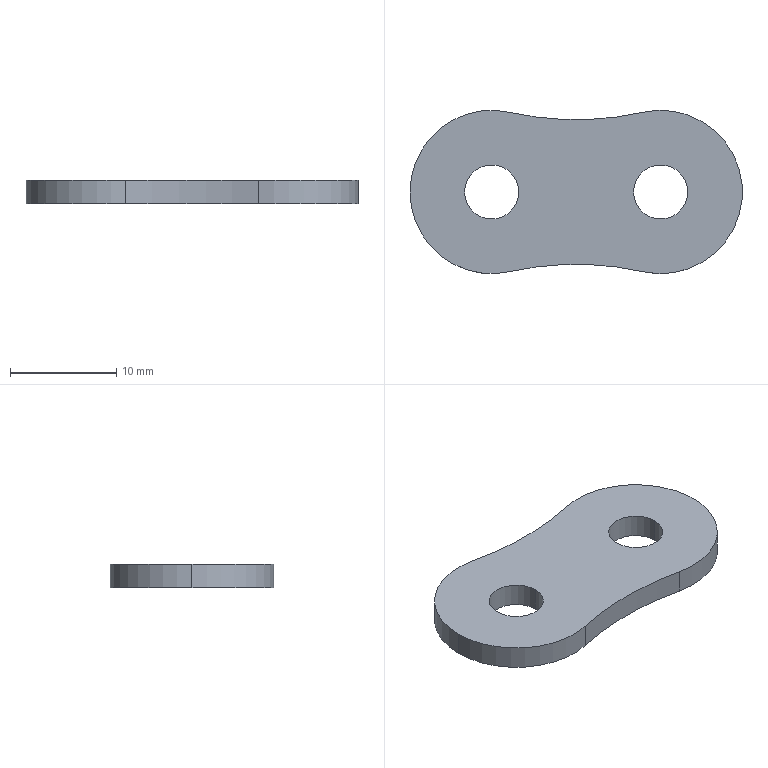Part | NX | features BREP 1 | 1 solid | 11 faces | box 31.225 x 15.35 x 2.22 mm | volume 824.256 mm3 | cylinder 9 | plane 2 | commonest cylinder face diameters 5.09 x4 15.35 x3 56.766 x2
STEP:
#1=CARTESIAN_POINT('',(5.393,0.,0.));
#2=VERTEX_POINT('',#1);
#3=CARTESIAN_POINT('',(10.482,0.,0.));
#4=VERTEX_POINT('',#3);
#5=CARTESIAN_POINT('',(7.938,0.,0.));
#6=DIRECTION('',(0.,0.,1.));
#7=DIRECTION('',(1.,0.,0.));
#8=AXIS2_PLACEMENT_3D('',#5,#6,#7);
#9=CIRCLE('',#8,2.545);
#10=EDGE_CURVE('',#2,#4,#9,.T.);
#11=ORIENTED_EDGE('',*,*,#10,.F.);
#12=CARTESIAN_POINT('',(5.393,0.,2.22));
#13=VERTEX_POINT('',#12);
#14=CARTESIAN_POINT('',(5.393,0.,0.));
#15=DIRECTION('',(0.,0.,1.));
#16=VECTOR('',#15,1000.);
#17=LINE('',#14,#16);
#18=EDGE_CURVE('',#13,#2,#17,.F.);
#19=ORIENTED_EDGE('',*,*,#18,.F.);
#20=CARTESIAN_POINT('',(10.482,0.,2.22));
#21=VERTEX_POINT('',#20);
#22=CARTESIAN_POINT('',(7.938,0.,2.22));
#23=DIRECTION('',(0.,0.,1.));
#24=DIRECTION('',(1.,0.,0.));
#25=AXIS2_PLACEMENT_3D('',#22,#23,#24);
#26=CIRCLE('',#25,2.545);
#27=EDGE_CURVE('',#13,#21,#26,.T.);
#28=ORIENTED_EDGE('',*,*,#27,.T.);
#29=CARTESIAN_POINT('',(10.482,0.,0.));
#30=DIRECTION('',(0.,0.,1.));
#31=VECTOR('',#30,1000.);
#32=LINE('',#29,#31);
#33=EDGE_CURVE('',#21,#4,#32,.F.);
#34=ORIENTED_EDGE('',*,*,#33,.T.);
#35=EDGE_LOOP('',(#11,#19,#28,#34));
#36=FACE_BOUND('',#35,.T.);
#37=CARTESIAN_POINT('',(7.938,0.,0.));
#38=DIRECTION('',(0.,0.,1.));
#39=DIRECTION('',(1.,0.,0.));
#40=AXIS2_PLACEMENT_3D('',#37,#38,#39);
#41=CYLINDRICAL_SURFACE('',#40,2.545);
#42=ADVANCED_FACE('',(#36),#41,.F.);
#43=CARTESIAN_POINT('',(-10.482,0.,0.));
#44=VERTEX_POINT('',#43);
#45=CARTESIAN_POINT('',(-5.393,0.,0.));
#46=VERTEX_POINT('',#45);
#47=CARTESIAN_POINT('',(-7.938,0.,0.));
#48=DIRECTION('',(0.,0.,1.));
#49=DIRECTION('',(1.,0.,0.));
#50=AXIS2_PLACEMENT_3D('',#47,#48,#49);
#51=CIRCLE('',#50,2.545);
#52=EDGE_CURVE('',#44,#46,#51,.T.);
#53=ORIENTED_EDGE('',*,*,#52,.F.);
#54=CARTESIAN_POINT('',(-10.482,0.,2.22));
#55=VERTEX_POINT('',#54);
#56=CARTESIAN_POINT('',(-10.482,0.,0.));
#57=DIRECTION('',(0.,0.,1.));
#58=VECTOR('',#57,1000.);
#59=LINE('',#56,#58);
#60=EDGE_CURVE('',#55,#44,#59,.F.);
#61=ORIENTED_EDGE('',*,*,#60,.F.);
#62=CARTESIAN_POINT('',(-5.393,0.,2.22));
#63=VERTEX_POINT('',#62);
#64=CARTESIAN_POINT('',(-7.938,0.,2.22));
#65=DIRECTION('',(0.,0.,1.));
#66=DIRECTION('',(1.,0.,0.));
#67=AXIS2_PLACEMENT_3D('',#64,#65,#66);
#68=CIRCLE('',#67,2.545);
#69=EDGE_CURVE('',#55,#63,#68,.T.);
#70=ORIENTED_EDGE('',*,*,#69,.T.);
#71=CARTESIAN_POINT('',(-5.393,0.,0.));
#72=DIRECTION('',(0.,0.,1.));
#73=VECTOR('',#72,1000.);
#74=LINE('',#71,#73);
#75=EDGE_CURVE('',#63,#46,#74,.F.);
#76=ORIENTED_EDGE('',*,*,#75,.T.);
#77=EDGE_LOOP('',(#53,#61,#70,#76));
#78=FACE_BOUND('',#77,.T.);
#79=CARTESIAN_POINT('',(-7.938,0.,0.));
#80=DIRECTION('',(0.,0.,1.));
#81=DIRECTION('',(1.,0.,0.));
#82=AXIS2_PLACEMENT_3D('',#79,#80,#81);
#83=CYLINDRICAL_SURFACE('',#82,2.545);
#84=ADVANCED_FACE('',(#78),#83,.F.);
#85=CARTESIAN_POINT('',(-15.613,0.,2.22));
#86=VERTEX_POINT('',#85);
#87=CARTESIAN_POINT('',(-6.248,-7.487,2.22));
#88=VERTEX_POINT('',#87);
#89=CARTESIAN_POINT('',(-7.938,0.,2.22));
#90=DIRECTION('',(0.,0.,1.));
#91=DIRECTION('',(1.,0.,0.));
#92=AXIS2_PLACEMENT_3D('',#89,#90,#91);
#93=CIRCLE('',#92,7.675);
#94=EDGE_CURVE('',#86,#88,#93,.T.);
#95=ORIENTED_EDGE('',*,*,#94,.F.);
#96=CARTESIAN_POINT('',(-15.613,0.,0.));
#97=VERTEX_POINT('',#96);
#98=CARTESIAN_POINT('',(-15.613,0.,2.22));
#99=DIRECTION('',(0.,0.,-1.));
#100=VECTOR('',#99,1000.);
#101=LINE('',#98,#100);
#102=EDGE_CURVE('',#86,#97,#101,.T.);
#103=ORIENTED_EDGE('',*,*,#102,.T.);
#104=CARTESIAN_POINT('',(-6.248,-7.487,0.));
#105=VERTEX_POINT('',#104);
#106=CARTESIAN_POINT('',(-7.938,0.,0.));
#107=DIRECTION('',(0.,0.,1.));
#108=DIRECTION('',(1.,0.,0.));
#109=AXIS2_PLACEMENT_3D('',#106,#107,#108);
#110=CIRCLE('',#109,7.675);
#111=EDGE_CURVE('',#97,#105,#110,.T.);
#112=ORIENTED_EDGE('',*,*,#111,.T.);
#113=CARTESIAN_POINT('',(-6.248,-7.487,2.22));
#114=DIRECTION('',(0.,0.,-1.));
#115=VECTOR('',#114,1000.);
#116=LINE('',#113,#115);
#117=EDGE_CURVE('',#88,#105,#116,.T.);
#118=ORIENTED_EDGE('',*,*,#117,.F.);
#119=EDGE_LOOP('',(#95,#103,#112,#118));
#120=FACE_BOUND('',#119,.T.);
#121=CARTESIAN_POINT('',(-7.938,0.,2.22));
#122=DIRECTION('',(0.,0.,-1.));
#123=DIRECTION('',(-1.,0.,0.));
#124=AXIS2_PLACEMENT_3D('',#121,#122,#123);
#125=CYLINDRICAL_SURFACE('',#124,7.675);
#126=ADVANCED_FACE('',(#120),#125,.T.);
#127=CARTESIAN_POINT('',(6.248,-7.487,0.));
#128=VERTEX_POINT('',#127);
#129=CARTESIAN_POINT('',(0.,-35.173,0.));
#130=DIRECTION('',(0.,0.,-1.));
#131=DIRECTION('',(1.,0.,0.));
#132=AXIS2_PLACEMENT_3D('',#129,#130,#131);
#133=CIRCLE('',#132,28.383);
#134=EDGE_CURVE('',#105,#128,#133,.T.);
#135=ORIENTED_EDGE('',*,*,#134,.T.);
#136=CARTESIAN_POINT('',(6.248,-7.487,2.22));
#137=VERTEX_POINT('',#136);
#138=CARTESIAN_POINT('',(6.248,-7.487,2.22));
#139=DIRECTION('',(0.,0.,-1.));
#140=VECTOR('',#139,1000.);
#141=LINE('',#138,#140);
#142=EDGE_CURVE('',#137,#128,#141,.T.);
#143=ORIENTED_EDGE('',*,*,#142,.F.);
#144=CARTESIAN_POINT('',(0.,-35.173,2.22));
#145=DIRECTION('',(0.,0.,-1.));
#146=DIRECTION('',(1.,0.,0.));
#147=AXIS2_PLACEMENT_3D('',#144,#145,#146);
#148=CIRCLE('',#147,28.383);
#149=EDGE_CURVE('',#88,#137,#148,.T.);
#150=ORIENTED_EDGE('',*,*,#149,.F.);
#151=ORIENTED_EDGE('',*,*,#117,.T.);
#152=EDGE_LOOP('',(#135,#143,#150,#151));
#153=FACE_BOUND('',#152,.T.);
#154=CARTESIAN_POINT('',(0.,-35.173,2.22));
#155=DIRECTION('',(0.,0.,-1.));
#156=DIRECTION('',(-1.,0.,0.));
#157=AXIS2_PLACEMENT_3D('',#154,#155,#156);
#158=CYLINDRICAL_SURFACE('',#157,28.383);
#159=ADVANCED_FACE('',(#153),#158,.F.);
#160=CARTESIAN_POINT('',(6.248,7.487,0.));
#161=VERTEX_POINT('',#160);
#162=CARTESIAN_POINT('',(7.938,0.,0.));
#163=DIRECTION('',(0.,0.,1.));
#164=DIRECTION('',(1.,0.,0.));
#165=AXIS2_PLACEMENT_3D('',#162,#163,#164);
#166=CIRCLE('',#165,7.675);
#167=EDGE_CURVE('',#128,#161,#166,.T.);
#168=ORIENTED_EDGE('',*,*,#167,.T.);
#169=CARTESIAN_POINT('',(6.248,7.487,2.22));
#170=VERTEX_POINT('',#169);
#171=CARTESIAN_POINT('',(6.248,7.487,2.22));
#172=DIRECTION('',(0.,0.,-1.));
#173=VECTOR('',#172,1000.);
#174=LINE('',#171,#173);
#175=EDGE_CURVE('',#170,#161,#174,.T.);
#176=ORIENTED_EDGE('',*,*,#175,.F.);
#177=CARTESIAN_POINT('',(7.938,0.,2.22));
#178=DIRECTION('',(0.,0.,1.));
#179=DIRECTION('',(1.,0.,0.));
#180=AXIS2_PLACEMENT_3D('',#177,#178,#179);
#181=CIRCLE('',#180,7.675);
#182=EDGE_CURVE('',#137,#170,#181,.T.);
#183=ORIENTED_EDGE('',*,*,#182,.F.);
#184=ORIENTED_EDGE('',*,*,#142,.T.);
#185=EDGE_LOOP('',(#168,#176,#183,#184));
#186=FACE_BOUND('',#185,.T.);
#187=CARTESIAN_POINT('',(7.938,0.,2.22));
#188=DIRECTION('',(0.,0.,-1.));
#189=DIRECTION('',(-1.,0.,0.));
#190=AXIS2_PLACEMENT_3D('',#187,#188,#189);
#191=CYLINDRICAL_SURFACE('',#190,7.675);
#192=ADVANCED_FACE('',(#186),#191,.T.);
#193=CARTESIAN_POINT('',(-6.248,7.487,0.));
#194=VERTEX_POINT('',#193);
#195=CARTESIAN_POINT('',(0.,35.173,0.));
#196=DIRECTION('',(0.,0.,-1.));
#197=DIRECTION('',(1.,0.,0.));
#198=AXIS2_PLACEMENT_3D('',#195,#196,#197);
#199=CIRCLE('',#198,28.383);
#200=EDGE_CURVE('',#161,#194,#199,.T.);
#201=ORIENTED_EDGE('',*,*,#200,.T.);
#202=CARTESIAN_POINT('',(-6.248,7.487,2.22));
#203=VERTEX_POINT('',#202);
#204=CARTESIAN_POINT('',(-6.248,7.487,2.22));
#205=DIRECTION('',(0.,0.,-1.));
#206=VECTOR('',#205,1000.);
#207=LINE('',#204,#206);
#208=EDGE_CURVE('',#203,#194,#207,.T.);
#209=ORIENTED_EDGE('',*,*,#208,.F.);
#210=CARTESIAN_POINT('',(0.,35.173,2.22));
#211=DIRECTION('',(0.,0.,-1.));
#212=DIRECTION('',(1.,0.,0.));
#213=AXIS2_PLACEMENT_3D('',#210,#211,#212);
#214=CIRCLE('',#213,28.383);
#215=EDGE_CURVE('',#170,#203,#214,.T.);
#216=ORIENTED_EDGE('',*,*,#215,.F.);
#217=ORIENTED_EDGE('',*,*,#175,.T.);
#218=EDGE_LOOP('',(#201,#209,#216,#217));
#219=FACE_BOUND('',#218,.T.);
#220=CARTESIAN_POINT('',(0.,35.173,2.22));
#221=DIRECTION('',(0.,0.,-1.));
#222=DIRECTION('',(-1.,0.,0.));
#223=AXIS2_PLACEMENT_3D('',#220,#221,#222);
#224=CYLINDRICAL_SURFACE('',#223,28.383);
#225=ADVANCED_FACE('',(#219),#224,.F.);
#226=ORIENTED_EDGE('',*,*,#102,.F.);
#227=CARTESIAN_POINT('',(-7.938,0.,2.22));
#228=DIRECTION('',(0.,0.,1.));
#229=DIRECTION('',(1.,0.,0.));
#230=AXIS2_PLACEMENT_3D('',#227,#228,#229);
#231=CIRCLE('',#230,7.675);
#232=EDGE_CURVE('',#203,#86,#231,.T.);
#233=ORIENTED_EDGE('',*,*,#232,.F.);
#234=ORIENTED_EDGE('',*,*,#208,.T.);
#235=CARTESIAN_POINT('',(-7.938,0.,0.));
#236=DIRECTION('',(0.,0.,1.));
#237=DIRECTION('',(1.,0.,0.));
#238=AXIS2_PLACEMENT_3D('',#235,#236,#237);
#239=CIRCLE('',#238,7.675);
#240=EDGE_CURVE('',#194,#97,#239,.T.);
#241=ORIENTED_EDGE('',*,*,#240,.T.);
#242=EDGE_LOOP('',(#226,#233,#234,#241));
#243=FACE_BOUND('',#242,.T.);
#244=CARTESIAN_POINT('',(-7.938,0.,2.22));
#245=DIRECTION('',(0.,0.,-1.));
#246=DIRECTION('',(-1.,0.,0.));
#247=AXIS2_PLACEMENT_3D('',#244,#245,#246);
#248=CYLINDRICAL_SURFACE('',#247,7.675);
#249=ADVANCED_FACE('',(#243),#248,.T.);
#250=ORIENTED_EDGE('',*,*,#149,.T.);
#251=ORIENTED_EDGE('',*,*,#182,.T.);
#252=ORIENTED_EDGE('',*,*,#215,.T.);
#253=ORIENTED_EDGE('',*,*,#232,.T.);
#254=ORIENTED_EDGE('',*,*,#94,.T.);
#255=EDGE_LOOP('',(#250,#251,#252,#253,#254));
#256=FACE_BOUND('',#255,.T.);
#257=CARTESIAN_POINT('',(7.938,0.,2.22));
#258=DIRECTION('',(0.,0.,1.));
#259=DIRECTION('',(1.,0.,0.));
#260=AXIS2_PLACEMENT_3D('',#257,#258,#259);
#261=CIRCLE('',#260,2.545);
#262=EDGE_CURVE('',#21,#13,#261,.T.);
#263=ORIENTED_EDGE('',*,*,#262,.F.);
#264=ORIENTED_EDGE('',*,*,#27,.F.);
#265=EDGE_LOOP('',(#263,#264));
#266=FACE_BOUND('',#265,.T.);
#267=CARTESIAN_POINT('',(-7.938,0.,2.22));
#268=DIRECTION('',(0.,0.,1.));
#269=DIRECTION('',(1.,0.,0.));
#270=AXIS2_PLACEMENT_3D('',#267,#268,#269);
#271=CIRCLE('',#270,2.545);
#272=EDGE_CURVE('',#63,#55,#271,.T.);
#273=ORIENTED_EDGE('',*,*,#272,.F.);
#274=ORIENTED_EDGE('',*,*,#69,.F.);
#275=EDGE_LOOP('',(#273,#274));
#276=FACE_BOUND('',#275,.T.);
#277=CARTESIAN_POINT('',(-3.969,-17.587,2.22));
#278=DIRECTION('',(0.,0.,1.));
#279=DIRECTION('',(1.,0.,0.));
#280=AXIS2_PLACEMENT_3D('',#277,#278,#279);
#281=PLANE('',#280);
#282=ADVANCED_FACE('',(#256,#266,#276),#281,.T.);
#283=ORIENTED_EDGE('',*,*,#134,.F.);
#284=ORIENTED_EDGE('',*,*,#111,.F.);
#285=ORIENTED_EDGE('',*,*,#240,.F.);
#286=ORIENTED_EDGE('',*,*,#200,.F.);
#287=ORIENTED_EDGE('',*,*,#167,.F.);
#288=EDGE_LOOP('',(#283,#284,#285,#286,#287));
#289=FACE_BOUND('',#288,.T.);
#290=CARTESIAN_POINT('',(7.938,0.,0.));
#291=DIRECTION('',(0.,0.,1.));
#292=DIRECTION('',(1.,0.,0.));
#293=AXIS2_PLACEMENT_3D('',#290,#291,#292);
#294=CIRCLE('',#293,2.545);
#295=EDGE_CURVE('',#4,#2,#294,.T.);
#296=ORIENTED_EDGE('',*,*,#295,.T.);
#297=ORIENTED_EDGE('',*,*,#10,.T.);
#298=EDGE_LOOP('',(#296,#297));
#299=FACE_BOUND('',#298,.T.);
#300=CARTESIAN_POINT('',(-7.938,0.,0.));
#301=DIRECTION('',(0.,0.,1.));
#302=DIRECTION('',(1.,0.,0.));
#303=AXIS2_PLACEMENT_3D('',#300,#301,#302);
#304=CIRCLE('',#303,2.545);
#305=EDGE_CURVE('',#46,#44,#304,.T.);
#306=ORIENTED_EDGE('',*,*,#305,.T.);
#307=ORIENTED_EDGE('',*,*,#52,.T.);
#308=EDGE_LOOP('',(#306,#307));
#309=FACE_BOUND('',#308,.T.);
#310=CARTESIAN_POINT('',(-3.969,-17.587,0.));
#311=DIRECTION('',(0.,0.,1.));
#312=DIRECTION('',(1.,0.,0.));
#313=AXIS2_PLACEMENT_3D('',#310,#311,#312);
#314=PLANE('',#313);
#315=ADVANCED_FACE('',(#289,#299,#309),#314,.F.);
#316=ORIENTED_EDGE('',*,*,#60,.T.);
#317=ORIENTED_EDGE('',*,*,#305,.F.);
#318=ORIENTED_EDGE('',*,*,#75,.F.);
#319=ORIENTED_EDGE('',*,*,#272,.T.);
#320=EDGE_LOOP('',(#316,#317,#318,#319));
#321=FACE_BOUND('',#320,.T.);
#322=CARTESIAN_POINT('',(-7.938,0.,0.));
#323=DIRECTION('',(0.,0.,1.));
#324=DIRECTION('',(1.,0.,0.));
#325=AXIS2_PLACEMENT_3D('',#322,#323,#324);
#326=CYLINDRICAL_SURFACE('',#325,2.545);
#327=ADVANCED_FACE('',(#321),#326,.F.);
#328=ORIENTED_EDGE('',*,*,#18,.T.);
#329=ORIENTED_EDGE('',*,*,#295,.F.);
#330=ORIENTED_EDGE('',*,*,#33,.F.);
#331=ORIENTED_EDGE('',*,*,#262,.T.);
#332=EDGE_LOOP('',(#328,#329,#330,#331));
#333=FACE_BOUND('',#332,.T.);
#334=CARTESIAN_POINT('',(7.938,0.,0.));
#335=DIRECTION('',(0.,0.,1.));
#336=DIRECTION('',(1.,0.,0.));
#337=AXIS2_PLACEMENT_3D('',#334,#335,#336);
#338=CYLINDRICAL_SURFACE('',#337,2.545);
#339=ADVANCED_FACE('',(#333),#338,.F.);
#340=CLOSED_SHELL('',(#42,#84,#126,#159,#192,#225,#249,#282,#315,#327,#339));
#341=MANIFOLD_SOLID_BREP('',#340);
#342=(LENGTH_UNIT()NAMED_UNIT(*)SI_UNIT(.MILLI.,.METRE.));
#343=UNCERTAINTY_MEASURE_WITH_UNIT(LENGTH_MEASURE(0.00001),#342,'','');
#344=(NAMED_UNIT(*)PLANE_ANGLE_UNIT()SI_UNIT($,.RADIAN.));
#345=(NAMED_UNIT(*)SI_UNIT($,.STERADIAN.)SOLID_ANGLE_UNIT());
#346=(GEOMETRIC_REPRESENTATION_CONTEXT(3)GLOBAL_UNCERTAINTY_ASSIGNED_CONTEXT((#343))GLOBAL_UNIT_ASSIGNED_CONTEXT((#342,#344,#345))REPRESENTATION_CONTEXT('',''));
#347=ADVANCED_BREP_SHAPE_REPRESENTATION('',(#341),#346);